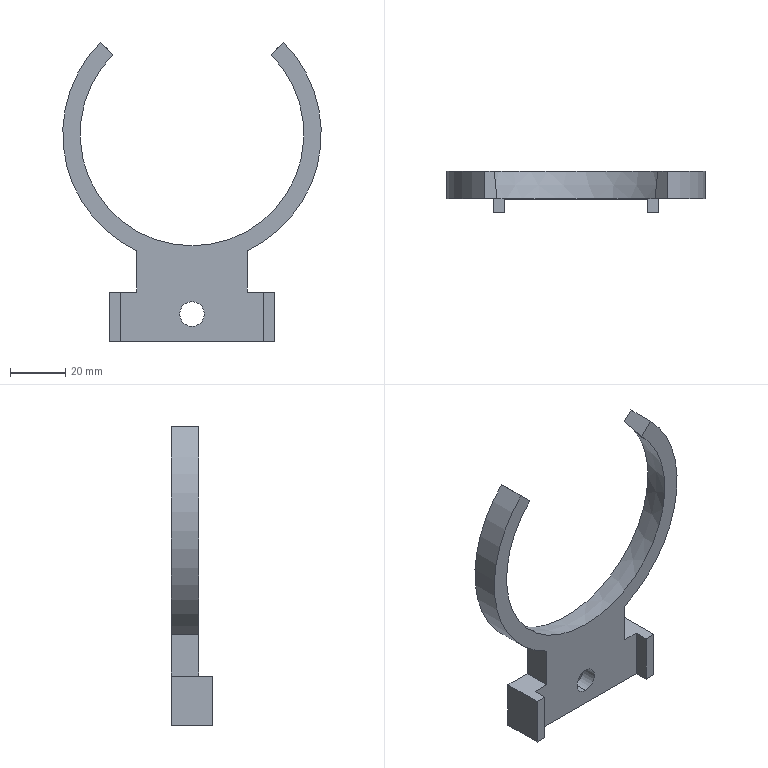Part | STEP file | Cup gripper V1.201001 | 1 solid | 22 faces | box 94 x 15 x 108.734 mm | volume 27097 mm3 | plane 15 | cylinder 4 | cone 3 | commonest cylinder face diameters 9 x2 94 x2